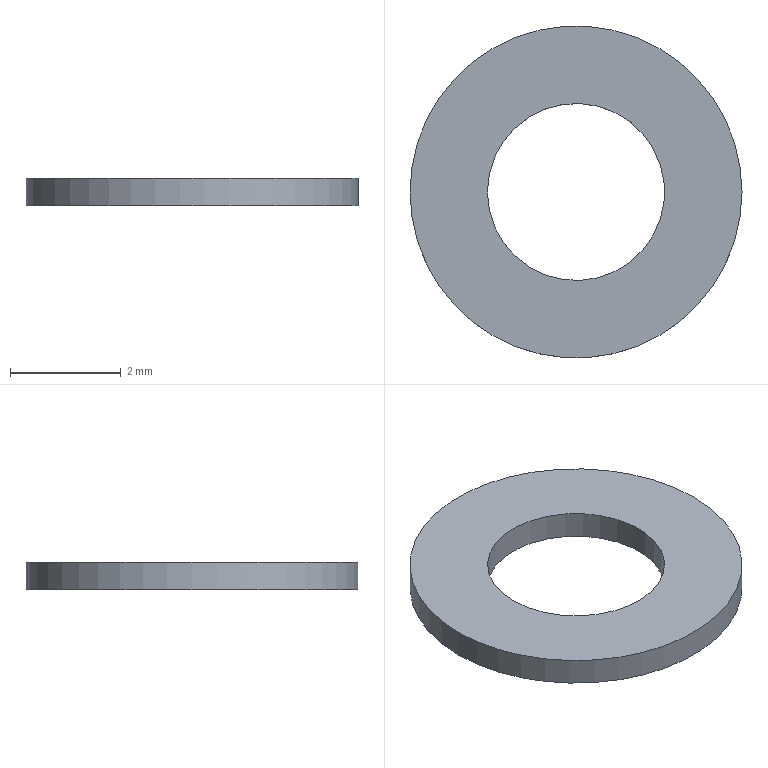Part | STEP file | 1 solid | 4 faces | box 6 x 6 x 0.5 mm | volume 10.116 mm3 | plane 2 | cylinder 2 | commonest cylinder face diameters 3.2 x1 6 x1
STEP:
#1=CARTESIAN_POINT('',(0.,0.,0.));
#2=DIRECTION('',(0.,0.,1.));
#3=DIRECTION('',(1.,0.,0.));
#4=AXIS2_PLACEMENT_3D('',#1,#2,#3);
#5=CARTESIAN_POINT('',(-1.6,0.,0.25));
#6=VERTEX_POINT('',#5);
#7=CARTESIAN_POINT('',(0.,0.,0.25));
#8=DIRECTION('',(0.,0.,1.));
#9=DIRECTION('',(-1.,0.,0.));
#10=AXIS2_PLACEMENT_3D('',#7,#8,#9);
#11=CIRCLE('',#10,1.6);
#12=CARTESIAN_POINT('',(0.,0.,0.25));
#13=DIRECTION('',(0.,0.,-1.));
#14=DIRECTION('',(-1.,0.,0.));
#15=AXIS2_PLACEMENT_3D('',#12,#13,#14);
#16=PLANE('',#15);
#17=CARTESIAN_POINT('',(1.6,0.));
#18=CARTESIAN_POINT('',(1.6,-2.771));
#19=CARTESIAN_POINT('',(-0.8,-1.386));
#20=CARTESIAN_POINT('',(-3.2,0.));
#21=CARTESIAN_POINT('',(-0.8,1.386));
#22=CARTESIAN_POINT('',(1.6,2.771));
#23=CARTESIAN_POINT('',(1.6,0.));
#24=(BOUNDED_CURVE()B_SPLINE_CURVE(2,(#17,#18,#19,#20,#21,#22,#23),.UNSPECIFIED.,.T.,.F.)B_SPLINE_CURVE_WITH_KNOTS((1,2,2,2,2,1),(-2.094,0.,2.094,4.189,6.283,8.378),.UNSPECIFIED.)CURVE()GEOMETRIC_REPRESENTATION_ITEM()RATIONAL_B_SPLINE_CURVE((1.,0.5,1.,0.5,1.,0.5,1.))REPRESENTATION_ITEM(''));
#25=(GEOMETRIC_REPRESENTATION_CONTEXT(2)PARAMETRIC_REPRESENTATION_CONTEXT()REPRESENTATION_CONTEXT('',''));
#26=DEFINITIONAL_REPRESENTATION('',(#24),#25);
#27=PCURVE('',#16,#26);
#28=CARTESIAN_POINT('',(0.,0.,0.275));
#29=DIRECTION('',(0.,0.,-1.));
#30=DIRECTION('',(-1.,0.,0.));
#31=AXIS2_PLACEMENT_3D('',#28,#29,#30);
#32=CYLINDRICAL_SURFACE('',#31,1.6);
#33=CARTESIAN_POINT('',(6.283,0.025));
#34=DIRECTION('',(-1.,0.));
#35=VECTOR('',#34,1.);
#36=LINE('',#33,#35);
#37=(GEOMETRIC_REPRESENTATION_CONTEXT(2)PARAMETRIC_REPRESENTATION_CONTEXT()REPRESENTATION_CONTEXT('',''));
#38=DEFINITIONAL_REPRESENTATION('',(#36),#37);
#39=PCURVE('',#32,#38);
#40=SURFACE_CURVE('',#11,(#27,#39),.PCURVE_S1.);
#41=EDGE_CURVE('',#6,#6,#40,.T.);
#42=ORIENTED_EDGE('',*,*,#41,.F.);
#43=EDGE_LOOP('',(#42));
#44=FACE_BOUND('',#43,.T.);
#45=CARTESIAN_POINT('',(-3.,0.,0.25));
#46=VERTEX_POINT('',#45);
#47=CARTESIAN_POINT('',(0.,0.,0.25));
#48=DIRECTION('',(0.,0.,-1.));
#49=DIRECTION('',(-1.,0.,0.));
#50=AXIS2_PLACEMENT_3D('',#47,#48,#49);
#51=CIRCLE('',#50,3.);
#52=CARTESIAN_POINT('',(0.,0.));
#53=DIRECTION('',(1.,0.));
#54=AXIS2_PLACEMENT_2D('',#52,#53);
#55=CIRCLE('',#54,3.);
#56=(GEOMETRIC_REPRESENTATION_CONTEXT(2)PARAMETRIC_REPRESENTATION_CONTEXT()REPRESENTATION_CONTEXT('',''));
#57=DEFINITIONAL_REPRESENTATION('',(#55),#56);
#58=PCURVE('',#16,#57);
#59=CARTESIAN_POINT('',(0.,0.,0.275));
#60=DIRECTION('',(0.,0.,-1.));
#61=DIRECTION('',(-1.,0.,0.));
#62=AXIS2_PLACEMENT_3D('',#59,#60,#61);
#63=CYLINDRICAL_SURFACE('',#62,3.);
#64=CARTESIAN_POINT('',(0.,0.025));
#65=DIRECTION('',(1.,0.));
#66=VECTOR('',#65,1.);
#67=LINE('',#64,#66);
#68=(GEOMETRIC_REPRESENTATION_CONTEXT(2)PARAMETRIC_REPRESENTATION_CONTEXT()REPRESENTATION_CONTEXT('',''));
#69=DEFINITIONAL_REPRESENTATION('',(#67),#68);
#70=PCURVE('',#63,#69);
#71=SURFACE_CURVE('',#51,(#58,#70),.PCURVE_S1.);
#72=EDGE_CURVE('',#46,#46,#71,.T.);
#73=ORIENTED_EDGE('',*,*,#72,.F.);
#74=EDGE_LOOP('',(#73));
#75=FACE_BOUND('',#74,.T.);
#76=ADVANCED_FACE('',(#44,#75),#16,.F.);
#77=CARTESIAN_POINT('',(-1.6,0.,-0.25));
#78=VERTEX_POINT('',#77);
#79=CARTESIAN_POINT('',(0.,0.,-0.25));
#80=DIRECTION('',(0.,0.,1.));
#81=DIRECTION('',(-1.,0.,0.));
#82=AXIS2_PLACEMENT_3D('',#79,#80,#81);
#83=CIRCLE('',#82,1.6);
#84=CARTESIAN_POINT('',(6.283,0.525));
#85=DIRECTION('',(-1.,0.));
#86=VECTOR('',#85,1.);
#87=LINE('',#84,#86);
#88=(GEOMETRIC_REPRESENTATION_CONTEXT(2)PARAMETRIC_REPRESENTATION_CONTEXT()REPRESENTATION_CONTEXT('',''));
#89=DEFINITIONAL_REPRESENTATION('',(#87),#88);
#90=PCURVE('',#32,#89);
#91=CARTESIAN_POINT('',(0.,0.,-0.25));
#92=DIRECTION('',(0.,0.,-1.));
#93=DIRECTION('',(-1.,0.,0.));
#94=AXIS2_PLACEMENT_3D('',#91,#92,#93);
#95=PLANE('',#94);
#96=CARTESIAN_POINT('',(1.6,0.));
#97=CARTESIAN_POINT('',(1.6,-2.771));
#98=CARTESIAN_POINT('',(-0.8,-1.386));
#99=CARTESIAN_POINT('',(-3.2,0.));
#100=CARTESIAN_POINT('',(-0.8,1.386));
#101=CARTESIAN_POINT('',(1.6,2.771));
#102=CARTESIAN_POINT('',(1.6,0.));
#103=(BOUNDED_CURVE()B_SPLINE_CURVE(2,(#96,#97,#98,#99,#100,#101,#102),.UNSPECIFIED.,.T.,.F.)B_SPLINE_CURVE_WITH_KNOTS((1,2,2,2,2,1),(-2.094,0.,2.094,4.189,6.283,8.378),.UNSPECIFIED.)CURVE()GEOMETRIC_REPRESENTATION_ITEM()RATIONAL_B_SPLINE_CURVE((1.,0.5,1.,0.5,1.,0.5,1.))REPRESENTATION_ITEM(''));
#104=(GEOMETRIC_REPRESENTATION_CONTEXT(2)PARAMETRIC_REPRESENTATION_CONTEXT()REPRESENTATION_CONTEXT('',''));
#105=DEFINITIONAL_REPRESENTATION('',(#103),#104);
#106=PCURVE('',#95,#105);
#107=SURFACE_CURVE('',#83,(#90,#106),.PCURVE_S1.);
#108=EDGE_CURVE('',#78,#78,#107,.T.);
#109=ORIENTED_EDGE('',*,*,#108,.T.);
#110=CARTESIAN_POINT('',(-1.6,0.,0.25));
#111=CARTESIAN_POINT('',(-1.6,0.,-0.25));
#112=B_SPLINE_CURVE_WITH_KNOTS('',1,(#110,#111),.UNSPECIFIED.,.F.,.F.,(2,2),(0.025,0.525),.PIECEWISE_BEZIER_KNOTS.);
#113=CARTESIAN_POINT('',(0.,0.));
#114=DIRECTION('',(0.,1.));
#115=VECTOR('',#114,1.);
#116=LINE('',#113,#115);
#117=(GEOMETRIC_REPRESENTATION_CONTEXT(2)PARAMETRIC_REPRESENTATION_CONTEXT()REPRESENTATION_CONTEXT('',''));
#118=DEFINITIONAL_REPRESENTATION('',(#116),#117);
#119=PCURVE('',#32,#118);
#120=CARTESIAN_POINT('',(6.283,0.));
#121=DIRECTION('',(0.,1.));
#122=VECTOR('',#121,1.);
#123=LINE('',#120,#122);
#124=(GEOMETRIC_REPRESENTATION_CONTEXT(2)PARAMETRIC_REPRESENTATION_CONTEXT()REPRESENTATION_CONTEXT('',''));
#125=DEFINITIONAL_REPRESENTATION('',(#123),#124);
#126=PCURVE('',#32,#125);
#127=SEAM_CURVE('',#112,(#119,#126),.PCURVE_S1.);
#128=EDGE_CURVE('',#6,#78,#127,.T.);
#129=ORIENTED_EDGE('',*,*,#128,.F.);
#130=ORIENTED_EDGE('',*,*,#41,.F.);
#131=ORIENTED_EDGE('',*,*,#128,.T.);
#132=EDGE_LOOP('',(#109,#129,#130,#131));
#133=FACE_BOUND('',#132,.F.);
#134=ADVANCED_FACE('',(#133),#32,.F.);
#135=CARTESIAN_POINT('',(-3.,0.,-0.25));
#136=VERTEX_POINT('',#135);
#137=CARTESIAN_POINT('',(0.,0.,-0.25));
#138=DIRECTION('',(0.,0.,1.));
#139=DIRECTION('',(-1.,0.,0.));
#140=AXIS2_PLACEMENT_3D('',#137,#138,#139);
#141=CIRCLE('',#140,3.);
#142=CARTESIAN_POINT('',(6.283,0.525));
#143=DIRECTION('',(-1.,0.));
#144=VECTOR('',#143,1.);
#145=LINE('',#142,#144);
#146=(GEOMETRIC_REPRESENTATION_CONTEXT(2)PARAMETRIC_REPRESENTATION_CONTEXT()REPRESENTATION_CONTEXT('',''));
#147=DEFINITIONAL_REPRESENTATION('',(#145),#146);
#148=PCURVE('',#63,#147);
#149=CARTESIAN_POINT('',(3.,0.));
#150=CARTESIAN_POINT('',(3.,-5.196));
#151=CARTESIAN_POINT('',(-1.5,-2.598));
#152=CARTESIAN_POINT('',(-6.,0.));
#153=CARTESIAN_POINT('',(-1.5,2.598));
#154=CARTESIAN_POINT('',(3.,5.196));
#155=CARTESIAN_POINT('',(3.,0.));
#156=(BOUNDED_CURVE()B_SPLINE_CURVE(2,(#149,#150,#151,#152,#153,#154,#155),.UNSPECIFIED.,.T.,.F.)B_SPLINE_CURVE_WITH_KNOTS((1,2,2,2,2,1),(-2.094,0.,2.094,4.189,6.283,8.378),.UNSPECIFIED.)CURVE()GEOMETRIC_REPRESENTATION_ITEM()RATIONAL_B_SPLINE_CURVE((1.,0.5,1.,0.5,1.,0.5,1.))REPRESENTATION_ITEM(''));
#157=(GEOMETRIC_REPRESENTATION_CONTEXT(2)PARAMETRIC_REPRESENTATION_CONTEXT()REPRESENTATION_CONTEXT('',''));
#158=DEFINITIONAL_REPRESENTATION('',(#156),#157);
#159=PCURVE('',#95,#158);
#160=SURFACE_CURVE('',#141,(#148,#159),.PCURVE_S1.);
#161=EDGE_CURVE('',#136,#136,#160,.T.);
#162=ORIENTED_EDGE('',*,*,#161,.T.);
#163=CARTESIAN_POINT('',(-3.,0.,0.25));
#164=CARTESIAN_POINT('',(-3.,0.,-0.25));
#165=B_SPLINE_CURVE_WITH_KNOTS('',1,(#163,#164),.UNSPECIFIED.,.F.,.F.,(2,2),(0.025,0.525),.PIECEWISE_BEZIER_KNOTS.);
#166=CARTESIAN_POINT('',(0.,0.));
#167=DIRECTION('',(0.,1.));
#168=VECTOR('',#167,1.);
#169=LINE('',#166,#168);
#170=(GEOMETRIC_REPRESENTATION_CONTEXT(2)PARAMETRIC_REPRESENTATION_CONTEXT()REPRESENTATION_CONTEXT('',''));
#171=DEFINITIONAL_REPRESENTATION('',(#169),#170);
#172=PCURVE('',#63,#171);
#173=CARTESIAN_POINT('',(6.283,0.));
#174=DIRECTION('',(0.,1.));
#175=VECTOR('',#174,1.);
#176=LINE('',#173,#175);
#177=(GEOMETRIC_REPRESENTATION_CONTEXT(2)PARAMETRIC_REPRESENTATION_CONTEXT()REPRESENTATION_CONTEXT('',''));
#178=DEFINITIONAL_REPRESENTATION('',(#176),#177);
#179=PCURVE('',#63,#178);
#180=SEAM_CURVE('',#165,(#172,#179),.PCURVE_S1.);
#181=EDGE_CURVE('',#46,#136,#180,.T.);
#182=ORIENTED_EDGE('',*,*,#181,.F.);
#183=ORIENTED_EDGE('',*,*,#72,.T.);
#184=ORIENTED_EDGE('',*,*,#181,.T.);
#185=EDGE_LOOP('',(#162,#182,#183,#184));
#186=FACE_BOUND('',#185,.T.);
#187=ADVANCED_FACE('',(#186),#63,.T.);
#188=ORIENTED_EDGE('',*,*,#108,.T.);
#189=EDGE_LOOP('',(#188));
#190=FACE_BOUND('',#189,.T.);
#191=ORIENTED_EDGE('',*,*,#161,.F.);
#192=EDGE_LOOP('',(#191));
#193=FACE_BOUND('',#192,.T.);
#194=ADVANCED_FACE('',(#190,#193),#95,.T.);
#195=CLOSED_SHELL('',(#76,#134,#187,#194));
#196=MANIFOLD_SOLID_BREP('',#195);
#197=(LENGTH_UNIT()NAMED_UNIT(*)SI_UNIT(.MILLI.,.METRE.));
#198=UNCERTAINTY_MEASURE_WITH_UNIT(LENGTH_MEASURE(0.00001),#197,'','');
#199=(NAMED_UNIT(*)PLANE_ANGLE_UNIT()SI_UNIT($,.RADIAN.));
#200=(NAMED_UNIT(*)SI_UNIT($,.STERADIAN.)SOLID_ANGLE_UNIT());
#201=(GEOMETRIC_REPRESENTATION_CONTEXT(3)GLOBAL_UNCERTAINTY_ASSIGNED_CONTEXT((#198))GLOBAL_UNIT_ASSIGNED_CONTEXT((#197,#199,#200))REPRESENTATION_CONTEXT('',''));
#202=ADVANCED_BREP_SHAPE_REPRESENTATION('',(#4,#196),#201);